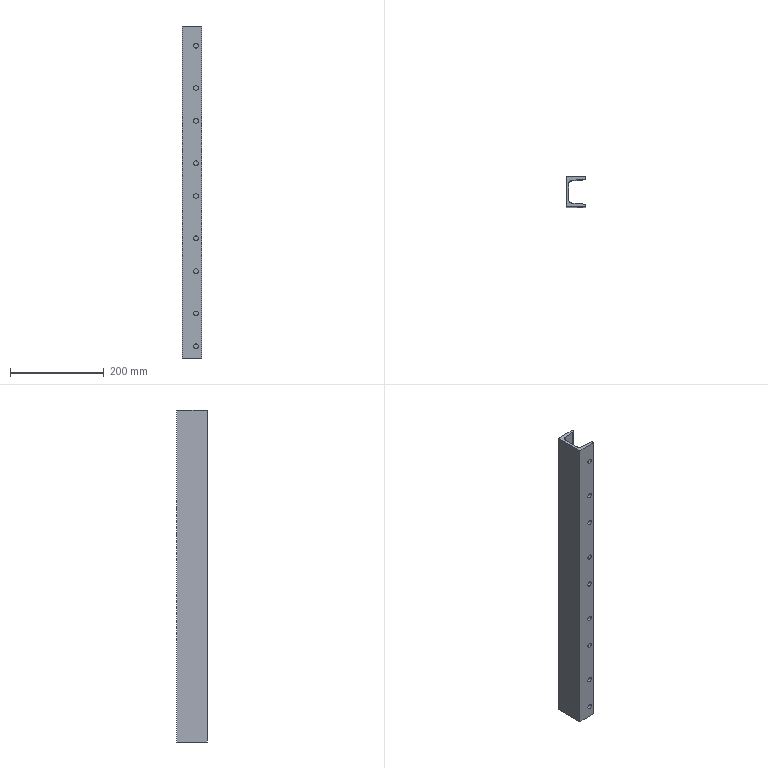Part | STEP file | DIN 1026-1 U 65 1785352380714 | 1 solid | 23 faces | box 42 x 65 x 707.157 mm | volume 633916 mm3 | cylinder 13 | plane 10 | commonest cylinder face diameters 10 x9 8 x2 15 x2
STEP:
#1=CARTESIAN_POINT('',(12.402,-24.312,60.));
#2=VERTEX_POINT('',#1);
#3=CARTESIAN_POINT('',(5.5,-16.836,60.));
#4=VERTEX_POINT('',#3);
#5=CARTESIAN_POINT('',(13.,-16.836,60.));
#6=DIRECTION('',(0.,0.,-1.));
#7=DIRECTION('',(-1.,0.,0.));
#8=AXIS2_PLACEMENT_3D('',#5,#6,#7);
#9=CIRCLE('',#8,7.5);
#10=EDGE_CURVE('',#2,#4,#9,.T.);
#11=ORIENTED_EDGE('',*,*,#10,.F.);
#12=CARTESIAN_POINT('',(38.319,-26.386,60.));
#13=VERTEX_POINT('',#12);
#14=CARTESIAN_POINT('',(15.707,-24.577,60.));
#15=DIRECTION('',(-0.9968,0.07975,0.));
#16=VECTOR('',#15,10.);
#17=LINE('',#14,#16);
#18=EDGE_CURVE('',#13,#2,#17,.T.);
#19=ORIENTED_EDGE('',*,*,#18,.F.);
#20=CARTESIAN_POINT('',(42.,-30.373,60.));
#21=VERTEX_POINT('',#20);
#22=CARTESIAN_POINT('',(38.,-30.373,60.));
#23=DIRECTION('',(0.,0.,1.));
#24=DIRECTION('',(-1.,0.,0.));
#25=AXIS2_PLACEMENT_3D('',#22,#23,#24);
#26=CIRCLE('',#25,4.);
#27=EDGE_CURVE('',#21,#13,#26,.T.);
#28=ORIENTED_EDGE('',*,*,#27,.F.);
#29=CARTESIAN_POINT('',(42.,-32.5,60.));
#30=VERTEX_POINT('',#29);
#31=CARTESIAN_POINT('',(42.,-15.186,60.));
#32=DIRECTION('',(0.,1.,0.));
#33=VECTOR('',#32,10.);
#34=LINE('',#31,#33);
#35=EDGE_CURVE('',#30,#21,#34,.T.);
#36=ORIENTED_EDGE('',*,*,#35,.F.);
#37=CARTESIAN_POINT('',(0.,-32.5,60.));
#38=VERTEX_POINT('',#37);
#39=CARTESIAN_POINT('',(31.5,-32.5,60.));
#40=DIRECTION('',(1.,0.,0.));
#41=VECTOR('',#40,10.);
#42=LINE('',#39,#41);
#43=EDGE_CURVE('',#38,#30,#42,.T.);
#44=ORIENTED_EDGE('',*,*,#43,.F.);
#45=CARTESIAN_POINT('',(0.,32.5,60.));
#46=VERTEX_POINT('',#45);
#47=CARTESIAN_POINT('',(0.,0.,60.));
#48=DIRECTION('',(0.,-1.,0.));
#49=VECTOR('',#48,10.);
#50=LINE('',#47,#49);
#51=EDGE_CURVE('',#46,#38,#50,.T.);
#52=ORIENTED_EDGE('',*,*,#51,.F.);
#53=CARTESIAN_POINT('',(42.,32.5,60.));
#54=VERTEX_POINT('',#53);
#55=CARTESIAN_POINT('',(10.5,32.5,60.));
#56=DIRECTION('',(-1.,0.,0.));
#57=VECTOR('',#56,10.);
#58=LINE('',#55,#57);
#59=EDGE_CURVE('',#54,#46,#58,.T.);
#60=ORIENTED_EDGE('',*,*,#59,.F.);
#61=CARTESIAN_POINT('',(42.,30.373,60.));
#62=VERTEX_POINT('',#61);
#63=CARTESIAN_POINT('',(42.,16.25,60.));
#64=DIRECTION('',(0.,1.,0.));
#65=VECTOR('',#64,10.);
#66=LINE('',#63,#65);
#67=EDGE_CURVE('',#62,#54,#66,.T.);
#68=ORIENTED_EDGE('',*,*,#67,.F.);
#69=CARTESIAN_POINT('',(38.319,26.386,60.));
#70=VERTEX_POINT('',#69);
#71=CARTESIAN_POINT('',(38.,30.373,60.));
#72=DIRECTION('',(0.,0.,1.));
#73=DIRECTION('',(-0.07975,0.9968,0.));
#74=AXIS2_PLACEMENT_3D('',#71,#72,#73);
#75=CIRCLE('',#74,4.);
#76=EDGE_CURVE('',#70,#62,#75,.T.);
#77=ORIENTED_EDGE('',*,*,#76,.F.);
#78=CARTESIAN_POINT('',(12.402,24.312,60.));
#79=VERTEX_POINT('',#78);
#80=CARTESIAN_POINT('',(28.666,25.613,60.));
#81=DIRECTION('',(0.9968,0.07975,0.));
#82=VECTOR('',#81,10.);
#83=LINE('',#80,#82);
#84=EDGE_CURVE('',#79,#70,#83,.T.);
#85=ORIENTED_EDGE('',*,*,#84,.F.);
#86=CARTESIAN_POINT('',(5.5,16.836,60.));
#87=VERTEX_POINT('',#86);
#88=CARTESIAN_POINT('',(13.,16.836,60.));
#89=DIRECTION('',(0.,0.,-1.));
#90=DIRECTION('',(-0.07975,0.9968,0.));
#91=AXIS2_PLACEMENT_3D('',#88,#89,#90);
#92=CIRCLE('',#91,7.5);
#93=EDGE_CURVE('',#87,#79,#92,.T.);
#94=ORIENTED_EDGE('',*,*,#93,.F.);
#95=CARTESIAN_POINT('',(5.5,0.,60.));
#96=DIRECTION('',(0.,1.,0.));
#97=VECTOR('',#96,10.);
#98=LINE('',#95,#97);
#99=EDGE_CURVE('',#4,#87,#98,.T.);
#100=ORIENTED_EDGE('',*,*,#99,.F.);
#101=EDGE_LOOP('',(#11,#19,#28,#36,#44,#52,#60,#68,#77,#85,#94,#100));
#102=FACE_OUTER_BOUND('',#101,.T.);
#103=CARTESIAN_POINT('',(21.,0.,60.));
#104=DIRECTION('',(0.,0.,-1.));
#105=DIRECTION('',(1.,0.,0.));
#106=AXIS2_PLACEMENT_3D('',#103,#104,#105);
#107=PLANE('',#106);
#108=ADVANCED_FACE('',(#102),#107,.T.);
#109=ORIENTED_EDGE('',*,*,#51,.T.);
#110=CARTESIAN_POINT('',(0.,-32.5,767.157));
#111=VERTEX_POINT('',#110);
#112=CARTESIAN_POINT('',(0.,-32.5,0.));
#113=DIRECTION('',(0.,0.,1.));
#114=VECTOR('',#113,10.);
#115=LINE('',#112,#114);
#116=EDGE_CURVE('',#38,#111,#115,.T.);
#117=ORIENTED_EDGE('',*,*,#116,.T.);
#118=CARTESIAN_POINT('',(0.,32.5,767.157));
#119=VERTEX_POINT('',#118);
#120=CARTESIAN_POINT('',(0.,0.,767.157));
#121=DIRECTION('',(0.,1.,0.));
#122=VECTOR('',#121,10.);
#123=LINE('',#120,#122);
#124=EDGE_CURVE('',#111,#119,#123,.T.);
#125=ORIENTED_EDGE('',*,*,#124,.T.);
#126=CARTESIAN_POINT('',(0.,32.5,0.));
#127=DIRECTION('',(0.,0.,1.));
#128=VECTOR('',#127,10.);
#129=LINE('',#126,#128);
#130=EDGE_CURVE('',#46,#119,#129,.T.);
#131=ORIENTED_EDGE('',*,*,#130,.F.);
#132=EDGE_LOOP('',(#109,#117,#125,#131));
#133=FACE_OUTER_BOUND('',#132,.T.);
#134=CARTESIAN_POINT('',(0.,0.,0.));
#135=DIRECTION('',(-1.,0.,0.));
#136=DIRECTION('',(0.,0.,1.));
#137=AXIS2_PLACEMENT_3D('',#134,#135,#136);
#138=PLANE('',#137);
#139=ADVANCED_FACE('',(#133),#138,.T.);
#140=ORIENTED_EDGE('',*,*,#43,.T.);
#141=CARTESIAN_POINT('',(42.,-32.5,767.157));
#142=VERTEX_POINT('',#141);
#143=CARTESIAN_POINT('',(42.,-32.5,0.));
#144=DIRECTION('',(0.,0.,1.));
#145=VECTOR('',#144,10.);
#146=LINE('',#143,#145);
#147=EDGE_CURVE('',#30,#142,#146,.T.);
#148=ORIENTED_EDGE('',*,*,#147,.T.);
#149=CARTESIAN_POINT('',(31.5,-32.5,767.157));
#150=DIRECTION('',(-1.,0.,0.));
#151=VECTOR('',#150,10.);
#152=LINE('',#149,#151);
#153=EDGE_CURVE('',#142,#111,#152,.T.);
#154=ORIENTED_EDGE('',*,*,#153,.T.);
#155=ORIENTED_EDGE('',*,*,#116,.F.);
#156=EDGE_LOOP('',(#140,#148,#154,#155));
#157=FACE_OUTER_BOUND('',#156,.T.);
#158=CARTESIAN_POINT('',(24.5,-32.5,155.));
#159=VERTEX_POINT('',#158);
#160=CARTESIAN_POINT('',(29.5,-32.5,155.));
#161=DIRECTION('',(0.,1.,0.));
#162=DIRECTION('',(1.,0.,0.));
#163=AXIS2_PLACEMENT_3D('',#160,#161,#162);
#164=CIRCLE('',#163,5.);
#165=EDGE_CURVE('',#159,#159,#164,.T.);
#166=ORIENTED_EDGE('',*,*,#165,.T.);
#167=EDGE_LOOP('',(#166));
#168=FACE_BOUND('',#167,.T.);
#169=CARTESIAN_POINT('',(24.5,-32.5,85.));
#170=VERTEX_POINT('',#169);
#171=CARTESIAN_POINT('',(29.5,-32.5,85.));
#172=DIRECTION('',(0.,1.,0.));
#173=DIRECTION('',(1.,0.,0.));
#174=AXIS2_PLACEMENT_3D('',#171,#172,#173);
#175=CIRCLE('',#174,5.);
#176=EDGE_CURVE('',#170,#170,#175,.T.);
#177=ORIENTED_EDGE('',*,*,#176,.T.);
#178=EDGE_LOOP('',(#177));
#179=FACE_BOUND('',#178,.T.);
#180=CARTESIAN_POINT('',(24.5,-32.5,315.));
#181=VERTEX_POINT('',#180);
#182=CARTESIAN_POINT('',(29.5,-32.5,315.));
#183=DIRECTION('',(0.,1.,0.));
#184=DIRECTION('',(1.,0.,0.));
#185=AXIS2_PLACEMENT_3D('',#182,#183,#184);
#186=CIRCLE('',#185,5.);
#187=EDGE_CURVE('',#181,#181,#186,.T.);
#188=ORIENTED_EDGE('',*,*,#187,.T.);
#189=EDGE_LOOP('',(#188));
#190=FACE_BOUND('',#189,.T.);
#191=CARTESIAN_POINT('',(24.5,-32.5,245.));
#192=VERTEX_POINT('',#191);
#193=CARTESIAN_POINT('',(29.5,-32.5,245.));
#194=DIRECTION('',(0.,1.,0.));
#195=DIRECTION('',(1.,0.,0.));
#196=AXIS2_PLACEMENT_3D('',#193,#194,#195);
#197=CIRCLE('',#196,5.);
#198=EDGE_CURVE('',#192,#192,#197,.T.);
#199=ORIENTED_EDGE('',*,*,#198,.T.);
#200=EDGE_LOOP('',(#199));
#201=FACE_BOUND('',#200,.T.);
#202=CARTESIAN_POINT('',(24.5,-32.5,475.));
#203=VERTEX_POINT('',#202);
#204=CARTESIAN_POINT('',(29.5,-32.5,475.));
#205=DIRECTION('',(0.,1.,0.));
#206=DIRECTION('',(1.,0.,0.));
#207=AXIS2_PLACEMENT_3D('',#204,#205,#206);
#208=CIRCLE('',#207,5.);
#209=EDGE_CURVE('',#203,#203,#208,.T.);
#210=ORIENTED_EDGE('',*,*,#209,.T.);
#211=EDGE_LOOP('',(#210));
#212=FACE_BOUND('',#211,.T.);
#213=CARTESIAN_POINT('',(24.5,-32.5,405.));
#214=VERTEX_POINT('',#213);
#215=CARTESIAN_POINT('',(29.5,-32.5,405.));
#216=DIRECTION('',(0.,1.,0.));
#217=DIRECTION('',(1.,0.,0.));
#218=AXIS2_PLACEMENT_3D('',#215,#216,#217);
#219=CIRCLE('',#218,5.);
#220=EDGE_CURVE('',#214,#214,#219,.T.);
#221=ORIENTED_EDGE('',*,*,#220,.T.);
#222=EDGE_LOOP('',(#221));
#223=FACE_BOUND('',#222,.T.);
#224=CARTESIAN_POINT('',(24.5,-32.5,635.));
#225=VERTEX_POINT('',#224);
#226=CARTESIAN_POINT('',(29.5,-32.5,635.));
#227=DIRECTION('',(0.,1.,0.));
#228=DIRECTION('',(1.,0.,0.));
#229=AXIS2_PLACEMENT_3D('',#226,#227,#228);
#230=CIRCLE('',#229,5.);
#231=EDGE_CURVE('',#225,#225,#230,.T.);
#232=ORIENTED_EDGE('',*,*,#231,.T.);
#233=EDGE_LOOP('',(#232));
#234=FACE_BOUND('',#233,.T.);
#235=CARTESIAN_POINT('',(24.5,-32.5,565.));
#236=VERTEX_POINT('',#235);
#237=CARTESIAN_POINT('',(29.5,-32.5,565.));
#238=DIRECTION('',(0.,1.,0.));
#239=DIRECTION('',(1.,0.,0.));
#240=AXIS2_PLACEMENT_3D('',#237,#238,#239);
#241=CIRCLE('',#240,5.);
#242=EDGE_CURVE('',#236,#236,#241,.T.);
#243=ORIENTED_EDGE('',*,*,#242,.T.);
#244=EDGE_LOOP('',(#243));
#245=FACE_BOUND('',#244,.T.);
#246=CARTESIAN_POINT('',(24.5,-32.5,725.));
#247=VERTEX_POINT('',#246);
#248=CARTESIAN_POINT('',(29.5,-32.5,725.));
#249=DIRECTION('',(0.,1.,0.));
#250=DIRECTION('',(1.,0.,0.));
#251=AXIS2_PLACEMENT_3D('',#248,#249,#250);
#252=CIRCLE('',#251,5.);
#253=EDGE_CURVE('',#247,#247,#252,.T.);
#254=ORIENTED_EDGE('',*,*,#253,.T.);
#255=EDGE_LOOP('',(#254));
#256=FACE_BOUND('',#255,.T.);
#257=CARTESIAN_POINT('',(42.,-32.5,0.));
#258=DIRECTION('',(0.,-1.,0.));
#259=DIRECTION('',(0.,0.,-1.));
#260=AXIS2_PLACEMENT_3D('',#257,#258,#259);
#261=PLANE('',#260);
#262=ADVANCED_FACE('',(#157,#168,#179,#190,#201,#212,#223,#234,#245,#256),#261,.T.);
#263=ORIENTED_EDGE('',*,*,#35,.T.);
#264=CARTESIAN_POINT('',(42.,-30.373,767.157));
#265=VERTEX_POINT('',#264);
#266=CARTESIAN_POINT('',(42.,-30.373,0.));
#267=DIRECTION('',(0.,0.,1.));
#268=VECTOR('',#267,10.);
#269=LINE('',#266,#268);
#270=EDGE_CURVE('',#21,#265,#269,.T.);
#271=ORIENTED_EDGE('',*,*,#270,.T.);
#272=CARTESIAN_POINT('',(42.,-15.186,767.157));
#273=DIRECTION('',(0.,-1.,0.));
#274=VECTOR('',#273,10.);
#275=LINE('',#272,#274);
#276=EDGE_CURVE('',#265,#142,#275,.T.);
#277=ORIENTED_EDGE('',*,*,#276,.T.);
#278=ORIENTED_EDGE('',*,*,#147,.F.);
#279=EDGE_LOOP('',(#263,#271,#277,#278));
#280=FACE_OUTER_BOUND('',#279,.T.);
#281=CARTESIAN_POINT('',(42.,-30.373,0.));
#282=DIRECTION('',(1.,0.,0.));
#283=DIRECTION('',(0.,0.,-1.));
#284=AXIS2_PLACEMENT_3D('',#281,#282,#283);
#285=PLANE('',#284);
#286=ADVANCED_FACE('',(#280),#285,.T.);
#287=ORIENTED_EDGE('',*,*,#27,.T.);
#288=CARTESIAN_POINT('',(38.319,-26.386,767.157));
#289=VERTEX_POINT('',#288);
#290=CARTESIAN_POINT('',(38.319,-26.386,0.));
#291=DIRECTION('',(0.,0.,1.));
#292=VECTOR('',#291,10.);
#293=LINE('',#290,#292);
#294=EDGE_CURVE('',#13,#289,#293,.T.);
#295=ORIENTED_EDGE('',*,*,#294,.T.);
#296=CARTESIAN_POINT('',(38.,-30.373,767.157));
#297=DIRECTION('',(0.,0.,-1.));
#298=DIRECTION('',(-1.,0.,0.));
#299=AXIS2_PLACEMENT_3D('',#296,#297,#298);
#300=CIRCLE('',#299,4.);
#301=EDGE_CURVE('',#289,#265,#300,.T.);
#302=ORIENTED_EDGE('',*,*,#301,.T.);
#303=ORIENTED_EDGE('',*,*,#270,.F.);
#304=EDGE_LOOP('',(#287,#295,#302,#303));
#305=FACE_OUTER_BOUND('',#304,.T.);
#306=CARTESIAN_POINT('',(38.,-30.373,0.));
#307=DIRECTION('',(0.,0.,1.));
#308=DIRECTION('',(-1.,0.,0.));
#309=AXIS2_PLACEMENT_3D('',#306,#307,#308);
#310=CYLINDRICAL_SURFACE('',#309,4.);
#311=ADVANCED_FACE('',(#305),#310,.T.);
#312=ORIENTED_EDGE('',*,*,#18,.T.);
#313=CARTESIAN_POINT('',(12.402,-24.312,767.157));
#314=VERTEX_POINT('',#313);
#315=CARTESIAN_POINT('',(12.402,-24.312,0.));
#316=DIRECTION('',(0.,0.,1.));
#317=VECTOR('',#316,10.);
#318=LINE('',#315,#317);
#319=EDGE_CURVE('',#2,#314,#318,.T.);
#320=ORIENTED_EDGE('',*,*,#319,.T.);
#321=CARTESIAN_POINT('',(15.707,-24.577,767.157));
#322=DIRECTION('',(0.9968,-0.07975,0.));
#323=VECTOR('',#322,10.);
#324=LINE('',#321,#323);
#325=EDGE_CURVE('',#314,#289,#324,.T.);
#326=ORIENTED_EDGE('',*,*,#325,.T.);
#327=ORIENTED_EDGE('',*,*,#294,.F.);
#328=EDGE_LOOP('',(#312,#320,#326,#327));
#329=FACE_OUTER_BOUND('',#328,.T.);
#330=CARTESIAN_POINT('',(24.5,-25.28,155.));
#331=VERTEX_POINT('',#330);
#332=CARTESIAN_POINT('',(29.5,-25.68,155.));
#333=DIRECTION('',(-0.07975,-0.9968,0.));
#334=DIRECTION('',(0.9968,-0.07975,0.));
#335=AXIS2_PLACEMENT_3D('',#332,#333,#334);
#336=ELLIPSE('',#335,5.016,5.);
#337=EDGE_CURVE('',#331,#331,#336,.T.);
#338=ORIENTED_EDGE('',*,*,#337,.T.);
#339=EDGE_LOOP('',(#338));
#340=FACE_BOUND('',#339,.T.);
#341=CARTESIAN_POINT('',(24.5,-25.28,85.));
#342=VERTEX_POINT('',#341);
#343=CARTESIAN_POINT('',(29.5,-25.68,85.));
#344=DIRECTION('',(-0.07975,-0.9968,0.));
#345=DIRECTION('',(0.9968,-0.07975,0.));
#346=AXIS2_PLACEMENT_3D('',#343,#344,#345);
#347=ELLIPSE('',#346,5.016,5.);
#348=EDGE_CURVE('',#342,#342,#347,.T.);
#349=ORIENTED_EDGE('',*,*,#348,.T.);
#350=EDGE_LOOP('',(#349));
#351=FACE_BOUND('',#350,.T.);
#352=CARTESIAN_POINT('',(24.5,-25.28,315.));
#353=VERTEX_POINT('',#352);
#354=CARTESIAN_POINT('',(29.5,-25.68,315.));
#355=DIRECTION('',(-0.07975,-0.9968,0.));
#356=DIRECTION('',(0.9968,-0.07975,0.));
#357=AXIS2_PLACEMENT_3D('',#354,#355,#356);
#358=ELLIPSE('',#357,5.016,5.);
#359=EDGE_CURVE('',#353,#353,#358,.T.);
#360=ORIENTED_EDGE('',*,*,#359,.T.);
#361=EDGE_LOOP('',(#360));
#362=FACE_BOUND('',#361,.T.);
#363=CARTESIAN_POINT('',(24.5,-25.28,245.));
#364=VERTEX_POINT('',#363);
#365=CARTESIAN_POINT('',(29.5,-25.68,245.));
#366=DIRECTION('',(-0.07975,-0.9968,0.));
#367=DIRECTION('',(0.9968,-0.07975,0.));
#368=AXIS2_PLACEMENT_3D('',#365,#366,#367);
#369=ELLIPSE('',#368,5.016,5.);
#370=EDGE_CURVE('',#364,#364,#369,.T.);
#371=ORIENTED_EDGE('',*,*,#370,.T.);
#372=EDGE_LOOP('',(#371));
#373=FACE_BOUND('',#372,.T.);
#374=CARTESIAN_POINT('',(24.5,-25.28,475.));
#375=VERTEX_POINT('',#374);
#376=CARTESIAN_POINT('',(29.5,-25.68,475.));
#377=DIRECTION('',(-0.07975,-0.9968,0.));
#378=DIRECTION('',(0.9968,-0.07975,0.));
#379=AXIS2_PLACEMENT_3D('',#376,#377,#378);
#380=ELLIPSE('',#379,5.016,5.);
#381=EDGE_CURVE('',#375,#375,#380,.T.);
#382=ORIENTED_EDGE('',*,*,#381,.T.);
#383=EDGE_LOOP('',(#382));
#384=FACE_BOUND('',#383,.T.);
#385=CARTESIAN_POINT('',(24.5,-25.28,405.));
#386=VERTEX_POINT('',#385);
#387=CARTESIAN_POINT('',(29.5,-25.68,405.));
#388=DIRECTION('',(-0.07975,-0.9968,0.));
#389=DIRECTION('',(0.9968,-0.07975,0.));
#390=AXIS2_PLACEMENT_3D('',#387,#388,#389);
#391=ELLIPSE('',#390,5.016,5.);
#392=EDGE_CURVE('',#386,#386,#391,.T.);
#393=ORIENTED_EDGE('',*,*,#392,.T.);
#394=EDGE_LOOP('',(#393));
#395=FACE_BOUND('',#394,.T.);
#396=CARTESIAN_POINT('',(24.5,-25.28,635.));
#397=VERTEX_POINT('',#396);
#398=CARTESIAN_POINT('',(29.5,-25.68,635.));
#399=DIRECTION('',(-0.07975,-0.9968,0.));
#400=DIRECTION('',(0.9968,-0.07975,0.));
#401=AXIS2_PLACEMENT_3D('',#398,#399,#400);
#402=ELLIPSE('',#401,5.016,5.);
#403=EDGE_CURVE('',#397,#397,#402,.T.);
#404=ORIENTED_EDGE('',*,*,#403,.T.);
#405=EDGE_LOOP('',(#404));
#406=FACE_BOUND('',#405,.T.);
#407=CARTESIAN_POINT('',(24.5,-25.28,565.));
#408=VERTEX_POINT('',#407);
#409=CARTESIAN_POINT('',(29.5,-25.68,565.));
#410=DIRECTION('',(-0.07975,-0.9968,0.));
#411=DIRECTION('',(0.9968,-0.07975,0.));
#412=AXIS2_PLACEMENT_3D('',#409,#410,#411);
#413=ELLIPSE('',#412,5.016,5.);
#414=EDGE_CURVE('',#408,#408,#413,.T.);
#415=ORIENTED_EDGE('',*,*,#414,.T.);
#416=EDGE_LOOP('',(#415));
#417=FACE_BOUND('',#416,.T.);
#418=CARTESIAN_POINT('',(24.5,-25.28,725.));
#419=VERTEX_POINT('',#418);
#420=CARTESIAN_POINT('',(29.5,-25.68,725.));
#421=DIRECTION('',(-0.07975,-0.9968,0.));
#422=DIRECTION('',(0.9968,-0.07975,0.));
#423=AXIS2_PLACEMENT_3D('',#420,#421,#422);
#424=ELLIPSE('',#423,5.016,5.);
#425=EDGE_CURVE('',#419,#419,#424,.T.);
#426=ORIENTED_EDGE('',*,*,#425,.T.);
#427=EDGE_LOOP('',(#426));
#428=FACE_BOUND('',#427,.T.);
#429=CARTESIAN_POINT('',(12.402,-24.312,0.));
#430=DIRECTION('',(0.07975,0.9968,0.));
#431=DIRECTION('',(0.,0.,1.));
#432=AXIS2_PLACEMENT_3D('',#429,#430,#431);
#433=PLANE('',#432);
#434=ADVANCED_FACE('',(#329,#340,#351,#362,#373,#384,#395,#406,#417,#428),#433,.T.);
#435=ORIENTED_EDGE('',*,*,#10,.T.);
#436=CARTESIAN_POINT('',(5.5,-16.836,767.157));
#437=VERTEX_POINT('',#436);
#438=CARTESIAN_POINT('',(5.5,-16.836,0.));
#439=DIRECTION('',(0.,0.,1.));
#440=VECTOR('',#439,10.);
#441=LINE('',#438,#440);
#442=EDGE_CURVE('',#4,#437,#441,.T.);
#443=ORIENTED_EDGE('',*,*,#442,.T.);
#444=CARTESIAN_POINT('',(13.,-16.836,767.157));
#445=DIRECTION('',(0.,0.,1.));
#446=DIRECTION('',(-1.,0.,0.));
#447=AXIS2_PLACEMENT_3D('',#444,#445,#446);
#448=CIRCLE('',#447,7.5);
#449=EDGE_CURVE('',#437,#314,#448,.T.);
#450=ORIENTED_EDGE('',*,*,#449,.T.);
#451=ORIENTED_EDGE('',*,*,#319,.F.);
#452=EDGE_LOOP('',(#435,#443,#450,#451));
#453=FACE_OUTER_BOUND('',#452,.T.);
#454=CARTESIAN_POINT('',(13.,-16.836,0.));
#455=DIRECTION('',(0.,0.,1.));
#456=DIRECTION('',(-1.,0.,0.));
#457=AXIS2_PLACEMENT_3D('',#454,#455,#456);
#458=CYLINDRICAL_SURFACE('',#457,7.5);
#459=ADVANCED_FACE('',(#453),#458,.F.);
#460=ORIENTED_EDGE('',*,*,#253,.F.);
#461=CARTESIAN_POINT('',(24.5,-32.5,725.));
#462=DIRECTION('',(0.,1.,0.));
#463=VECTOR('',#462,5.);
#464=LINE('',#461,#463);
#465=EDGE_CURVE('',#247,#419,#464,.T.);
#466=ORIENTED_EDGE('',*,*,#465,.T.);
#467=ORIENTED_EDGE('',*,*,#425,.F.);
#468=ORIENTED_EDGE('',*,*,#465,.F.);
#469=EDGE_LOOP('',(#460,#466,#467,#468));
#470=FACE_OUTER_BOUND('',#469,.T.);
#471=CARTESIAN_POINT('',(29.5,-32.5,725.));
#472=DIRECTION('',(0.,1.,0.));
#473=DIRECTION('',(1.,0.,0.));
#474=AXIS2_PLACEMENT_3D('',#471,#472,#473);
#475=CYLINDRICAL_SURFACE('',#474,5.);
#476=ADVANCED_FACE('',(#470),#475,.F.);
#477=ORIENTED_EDGE('',*,*,#242,.F.);
#478=CARTESIAN_POINT('',(24.5,-32.5,565.));
#479=DIRECTION('',(0.,1.,0.));
#480=VECTOR('',#479,5.);
#481=LINE('',#478,#480);
#482=EDGE_CURVE('',#236,#408,#481,.T.);
#483=ORIENTED_EDGE('',*,*,#482,.T.);
#484=ORIENTED_EDGE('',*,*,#414,.F.);
#485=ORIENTED_EDGE('',*,*,#482,.F.);
#486=EDGE_LOOP('',(#477,#483,#484,#485));
#487=FACE_OUTER_BOUND('',#486,.T.);
#488=CARTESIAN_POINT('',(29.5,-32.5,565.));
#489=DIRECTION('',(0.,1.,0.));
#490=DIRECTION('',(1.,0.,0.));
#491=AXIS2_PLACEMENT_3D('',#488,#489,#490);
#492=CYLINDRICAL_SURFACE('',#491,5.);
#493=ADVANCED_FACE('',(#487),#492,.F.);
#494=ORIENTED_EDGE('',*,*,#231,.F.);
#495=CARTESIAN_POINT('',(24.5,-32.5,635.));
#496=DIRECTION('',(0.,1.,0.));
#497=VECTOR('',#496,5.);
#498=LINE('',#495,#497);
#499=EDGE_CURVE('',#225,#397,#498,.T.);
#500=ORIENTED_EDGE('',*,*,#499,.T.);
#501=ORIENTED_EDGE('',*,*,#403,.F.);
#502=ORIENTED_EDGE('',*,*,#499,.F.);
#503=EDGE_LOOP('',(#494,#500,#501,#502));
#504=FACE_OUTER_BOUND('',#503,.T.);
#505=CARTESIAN_POINT('',(29.5,-32.5,635.));
#506=DIRECTION('',(0.,1.,0.));
#507=DIRECTION('',(1.,0.,0.));
#508=AXIS2_PLACEMENT_3D('',#505,#506,#507);
#509=CYLINDRICAL_SURFACE('',#508,5.);
#510=ADVANCED_FACE('',(#504),#509,.F.);
#511=ORIENTED_EDGE('',*,*,#220,.F.);
#512=CARTESIAN_POINT('',(24.5,-32.5,405.));
#513=DIRECTION('',(0.,1.,0.));
#514=VECTOR('',#513,5.);
#515=LINE('',#512,#514);
#516=EDGE_CURVE('',#214,#386,#515,.T.);
#517=ORIENTED_EDGE('',*,*,#516,.T.);
#518=ORIENTED_EDGE('',*,*,#392,.F.);
#519=ORIENTED_EDGE('',*,*,#516,.F.);
#520=EDGE_LOOP('',(#511,#517,#518,#519));
#521=FACE_OUTER_BOUND('',#520,.T.);
#522=CARTESIAN_POINT('',(29.5,-32.5,405.));
#523=DIRECTION('',(0.,1.,0.));
#524=DIRECTION('',(1.,0.,0.));
#525=AXIS2_PLACEMENT_3D('',#522,#523,#524);
#526=CYLINDRICAL_SURFACE('',#525,5.);
#527=ADVANCED_FACE('',(#521),#526,.F.);
#528=ORIENTED_EDGE('',*,*,#209,.F.);
#529=CARTESIAN_POINT('',(24.5,-32.5,475.));
#530=DIRECTION('',(0.,1.,0.));
#531=VECTOR('',#530,5.);
#532=LINE('',#529,#531);
#533=EDGE_CURVE('',#203,#375,#532,.T.);
#534=ORIENTED_EDGE('',*,*,#533,.T.);
#535=ORIENTED_EDGE('',*,*,#381,.F.);
#536=ORIENTED_EDGE('',*,*,#533,.F.);
#537=EDGE_LOOP('',(#528,#534,#535,#536));
#538=FACE_OUTER_BOUND('',#537,.T.);
#539=CARTESIAN_POINT('',(29.5,-32.5,475.));
#540=DIRECTION('',(0.,1.,0.));
#541=DIRECTION('',(1.,0.,0.));
#542=AXIS2_PLACEMENT_3D('',#539,#540,#541);
#543=CYLINDRICAL_SURFACE('',#542,5.);
#544=ADVANCED_FACE('',(#538),#543,.F.);
#545=ORIENTED_EDGE('',*,*,#198,.F.);
#546=CARTESIAN_POINT('',(24.5,-32.5,245.));
#547=DIRECTION('',(0.,1.,0.));
#548=VECTOR('',#547,5.);
#549=LINE('',#546,#548);
#550=EDGE_CURVE('',#192,#364,#549,.T.);
#551=ORIENTED_EDGE('',*,*,#550,.T.);
#552=ORIENTED_EDGE('',*,*,#370,.F.);
#553=ORIENTED_EDGE('',*,*,#550,.F.);
#554=EDGE_LOOP('',(#545,#551,#552,#553));
#555=FACE_OUTER_BOUND('',#554,.T.);
#556=CARTESIAN_POINT('',(29.5,-32.5,245.));
#557=DIRECTION('',(0.,1.,0.));
#558=DIRECTION('',(1.,0.,0.));
#559=AXIS2_PLACEMENT_3D('',#556,#557,#558);
#560=CYLINDRICAL_SURFACE('',#559,5.);
#561=ADVANCED_FACE('',(#555),#560,.F.);
#562=ORIENTED_EDGE('',*,*,#187,.F.);
#563=CARTESIAN_POINT('',(24.5,-32.5,315.));
#564=DIRECTION('',(0.,1.,0.));
#565=VECTOR('',#564,5.);
#566=LINE('',#563,#565);
#567=EDGE_CURVE('',#181,#353,#566,.T.);
#568=ORIENTED_EDGE('',*,*,#567,.T.);
#569=ORIENTED_EDGE('',*,*,#359,.F.);
#570=ORIENTED_EDGE('',*,*,#567,.F.);
#571=EDGE_LOOP('',(#562,#568,#569,#570));
#572=FACE_OUTER_BOUND('',#571,.T.);
#573=CARTESIAN_POINT('',(29.5,-32.5,315.));
#574=DIRECTION('',(0.,1.,0.));
#575=DIRECTION('',(1.,0.,0.));
#576=AXIS2_PLACEMENT_3D('',#573,#574,#575);
#577=CYLINDRICAL_SURFACE('',#576,5.);
#578=ADVANCED_FACE('',(#572),#577,.F.);
#579=ORIENTED_EDGE('',*,*,#176,.F.);
#580=CARTESIAN_POINT('',(24.5,-32.5,85.));
#581=DIRECTION('',(0.,1.,0.));
#582=VECTOR('',#581,5.);
#583=LINE('',#580,#582);
#584=EDGE_CURVE('',#170,#342,#583,.T.);
#585=ORIENTED_EDGE('',*,*,#584,.T.);
#586=ORIENTED_EDGE('',*,*,#348,.F.);
#587=ORIENTED_EDGE('',*,*,#584,.F.);
#588=EDGE_LOOP('',(#579,#585,#586,#587));
#589=FACE_OUTER_BOUND('',#588,.T.);
#590=CARTESIAN_POINT('',(29.5,-32.5,85.));
#591=DIRECTION('',(0.,1.,0.));
#592=DIRECTION('',(1.,0.,0.));
#593=AXIS2_PLACEMENT_3D('',#590,#591,#592);
#594=CYLINDRICAL_SURFACE('',#593,5.);
#595=ADVANCED_FACE('',(#589),#594,.F.);
#596=ORIENTED_EDGE('',*,*,#165,.F.);
#597=CARTESIAN_POINT('',(24.5,-32.5,155.));
#598=DIRECTION('',(0.,1.,0.));
#599=VECTOR('',#598,5.);
#600=LINE('',#597,#599);
#601=EDGE_CURVE('',#159,#331,#600,.T.);
#602=ORIENTED_EDGE('',*,*,#601,.T.);
#603=ORIENTED_EDGE('',*,*,#337,.F.);
#604=ORIENTED_EDGE('',*,*,#601,.F.);
#605=EDGE_LOOP('',(#596,#602,#603,#604));
#606=FACE_OUTER_BOUND('',#605,.T.);
#607=CARTESIAN_POINT('',(29.5,-32.5,155.));
#608=DIRECTION('',(0.,1.,0.));
#609=DIRECTION('',(1.,0.,0.));
#610=AXIS2_PLACEMENT_3D('',#607,#608,#609);
#611=CYLINDRICAL_SURFACE('',#610,5.);
#612=ADVANCED_FACE('',(#606),#611,.F.);
#613=ORIENTED_EDGE('',*,*,#59,.T.);
#614=ORIENTED_EDGE('',*,*,#130,.T.);
#615=CARTESIAN_POINT('',(42.,32.5,767.157));
#616=VERTEX_POINT('',#615);
#617=CARTESIAN_POINT('',(10.5,32.5,767.157));
#618=DIRECTION('',(1.,0.,0.));
#619=VECTOR('',#618,10.);
#620=LINE('',#617,#619);
#621=EDGE_CURVE('',#119,#616,#620,.T.);
#622=ORIENTED_EDGE('',*,*,#621,.T.);
#623=CARTESIAN_POINT('',(42.,32.5,0.));
#624=DIRECTION('',(0.,0.,1.));
#625=VECTOR('',#624,10.);
#626=LINE('',#623,#625);
#627=EDGE_CURVE('',#54,#616,#626,.T.);
#628=ORIENTED_EDGE('',*,*,#627,.F.);
#629=EDGE_LOOP('',(#613,#614,#622,#628));
#630=FACE_OUTER_BOUND('',#629,.T.);
#631=CARTESIAN_POINT('',(0.,32.5,0.));
#632=DIRECTION('',(0.,1.,0.));
#633=DIRECTION('',(0.,0.,1.));
#634=AXIS2_PLACEMENT_3D('',#631,#632,#633);
#635=PLANE('',#634);
#636=ADVANCED_FACE('',(#630),#635,.T.);
#637=ORIENTED_EDGE('',*,*,#67,.T.);
#638=ORIENTED_EDGE('',*,*,#627,.T.);
#639=CARTESIAN_POINT('',(42.,30.373,767.157));
#640=VERTEX_POINT('',#639);
#641=CARTESIAN_POINT('',(42.,16.25,767.157));
#642=DIRECTION('',(0.,-1.,0.));
#643=VECTOR('',#642,10.);
#644=LINE('',#641,#643);
#645=EDGE_CURVE('',#616,#640,#644,.T.);
#646=ORIENTED_EDGE('',*,*,#645,.T.);
#647=CARTESIAN_POINT('',(42.,30.373,0.));
#648=DIRECTION('',(0.,0.,1.));
#649=VECTOR('',#648,10.);
#650=LINE('',#647,#649);
#651=EDGE_CURVE('',#62,#640,#650,.T.);
#652=ORIENTED_EDGE('',*,*,#651,.F.);
#653=EDGE_LOOP('',(#637,#638,#646,#652));
#654=FACE_OUTER_BOUND('',#653,.T.);
#655=CARTESIAN_POINT('',(42.,32.5,0.));
#656=DIRECTION('',(1.,0.,0.));
#657=DIRECTION('',(0.,0.,-1.));
#658=AXIS2_PLACEMENT_3D('',#655,#656,#657);
#659=PLANE('',#658);
#660=ADVANCED_FACE('',(#654),#659,.T.);
#661=ORIENTED_EDGE('',*,*,#76,.T.);
#662=ORIENTED_EDGE('',*,*,#651,.T.);
#663=CARTESIAN_POINT('',(38.319,26.386,767.157));
#664=VERTEX_POINT('',#663);
#665=CARTESIAN_POINT('',(38.,30.373,767.157));
#666=DIRECTION('',(0.,0.,-1.));
#667=DIRECTION('',(-0.07975,0.9968,0.));
#668=AXIS2_PLACEMENT_3D('',#665,#666,#667);
#669=CIRCLE('',#668,4.);
#670=EDGE_CURVE('',#640,#664,#669,.T.);
#671=ORIENTED_EDGE('',*,*,#670,.T.);
#672=CARTESIAN_POINT('',(38.319,26.386,0.));
#673=DIRECTION('',(0.,0.,1.));
#674=VECTOR('',#673,10.);
#675=LINE('',#672,#674);
#676=EDGE_CURVE('',#70,#664,#675,.T.);
#677=ORIENTED_EDGE('',*,*,#676,.F.);
#678=EDGE_LOOP('',(#661,#662,#671,#677));
#679=FACE_OUTER_BOUND('',#678,.T.);
#680=CARTESIAN_POINT('',(38.,30.373,0.));
#681=DIRECTION('',(0.,0.,1.));
#682=DIRECTION('',(-0.07975,0.9968,0.));
#683=AXIS2_PLACEMENT_3D('',#680,#681,#682);
#684=CYLINDRICAL_SURFACE('',#683,4.);
#685=ADVANCED_FACE('',(#679),#684,.T.);
#686=ORIENTED_EDGE('',*,*,#84,.T.);
#687=ORIENTED_EDGE('',*,*,#676,.T.);
#688=CARTESIAN_POINT('',(12.402,24.312,767.157));
#689=VERTEX_POINT('',#688);
#690=CARTESIAN_POINT('',(28.666,25.613,767.157));
#691=DIRECTION('',(-0.9968,-0.07975,0.));
#692=VECTOR('',#691,10.);
#693=LINE('',#690,#692);
#694=EDGE_CURVE('',#664,#689,#693,.T.);
#695=ORIENTED_EDGE('',*,*,#694,.T.);
#696=CARTESIAN_POINT('',(12.402,24.312,0.));
#697=DIRECTION('',(0.,0.,1.));
#698=VECTOR('',#697,10.);
#699=LINE('',#696,#698);
#700=EDGE_CURVE('',#79,#689,#699,.T.);
#701=ORIENTED_EDGE('',*,*,#700,.F.);
#702=EDGE_LOOP('',(#686,#687,#695,#701));
#703=FACE_OUTER_BOUND('',#702,.T.);
#704=CARTESIAN_POINT('',(38.319,26.386,0.));
#705=DIRECTION('',(0.07975,-0.9968,0.));
#706=DIRECTION('',(0.,0.,-1.));
#707=AXIS2_PLACEMENT_3D('',#704,#705,#706);
#708=PLANE('',#707);
#709=ADVANCED_FACE('',(#703),#708,.T.);
#710=ORIENTED_EDGE('',*,*,#93,.T.);
#711=ORIENTED_EDGE('',*,*,#700,.T.);
#712=CARTESIAN_POINT('',(5.5,16.836,767.157));
#713=VERTEX_POINT('',#712);
#714=CARTESIAN_POINT('',(13.,16.836,767.157));
#715=DIRECTION('',(0.,0.,1.));
#716=DIRECTION('',(-0.07975,0.9968,0.));
#717=AXIS2_PLACEMENT_3D('',#714,#715,#716);
#718=CIRCLE('',#717,7.5);
#719=EDGE_CURVE('',#689,#713,#718,.T.);
#720=ORIENTED_EDGE('',*,*,#719,.T.);
#721=CARTESIAN_POINT('',(5.5,16.836,0.));
#722=DIRECTION('',(0.,0.,1.));
#723=VECTOR('',#722,10.);
#724=LINE('',#721,#723);
#725=EDGE_CURVE('',#87,#713,#724,.T.);
#726=ORIENTED_EDGE('',*,*,#725,.F.);
#727=EDGE_LOOP('',(#710,#711,#720,#726));
#728=FACE_OUTER_BOUND('',#727,.T.);
#729=CARTESIAN_POINT('',(13.,16.836,0.));
#730=DIRECTION('',(0.,0.,1.));
#731=DIRECTION('',(-0.07975,0.9968,0.));
#732=AXIS2_PLACEMENT_3D('',#729,#730,#731);
#733=CYLINDRICAL_SURFACE('',#732,7.5);
#734=ADVANCED_FACE('',(#728),#733,.F.);
#735=ORIENTED_EDGE('',*,*,#99,.T.);
#736=ORIENTED_EDGE('',*,*,#725,.T.);
#737=CARTESIAN_POINT('',(5.5,0.,767.157));
#738=DIRECTION('',(0.,-1.,0.));
#739=VECTOR('',#738,10.);
#740=LINE('',#737,#739);
#741=EDGE_CURVE('',#713,#437,#740,.T.);
#742=ORIENTED_EDGE('',*,*,#741,.T.);
#743=ORIENTED_EDGE('',*,*,#442,.F.);
#744=EDGE_LOOP('',(#735,#736,#742,#743));
#745=FACE_OUTER_BOUND('',#744,.T.);
#746=CARTESIAN_POINT('',(5.5,0.,0.));
#747=DIRECTION('',(1.,0.,0.));
#748=DIRECTION('',(0.,0.,-1.));
#749=AXIS2_PLACEMENT_3D('',#746,#747,#748);
#750=PLANE('',#749);
#751=ADVANCED_FACE('',(#745),#750,.T.);
#752=ORIENTED_EDGE('',*,*,#621,.F.);
#753=ORIENTED_EDGE('',*,*,#124,.F.);
#754=ORIENTED_EDGE('',*,*,#153,.F.);
#755=ORIENTED_EDGE('',*,*,#276,.F.);
#756=ORIENTED_EDGE('',*,*,#301,.F.);
#757=ORIENTED_EDGE('',*,*,#325,.F.);
#758=ORIENTED_EDGE('',*,*,#449,.F.);
#759=ORIENTED_EDGE('',*,*,#741,.F.);
#760=ORIENTED_EDGE('',*,*,#719,.F.);
#761=ORIENTED_EDGE('',*,*,#694,.F.);
#762=ORIENTED_EDGE('',*,*,#670,.F.);
#763=ORIENTED_EDGE('',*,*,#645,.F.);
#764=EDGE_LOOP('',(#752,#753,#754,#755,#756,#757,#758,#759,#760,#761,#762,#763));
#765=FACE_OUTER_BOUND('',#764,.T.);
#766=CARTESIAN_POINT('',(21.,0.,767.157));
#767=DIRECTION('',(0.,0.,1.));
#768=DIRECTION('',(1.,0.,0.));
#769=AXIS2_PLACEMENT_3D('',#766,#767,#768);
#770=PLANE('',#769);
#771=ADVANCED_FACE('',(#765),#770,.T.);
#772=CLOSED_SHELL('',(#108,#139,#262,#286,#311,#434,#459,#476,#493,#510,#527,#544,#561,#578,#595,#612,#636,#660,#685,#709,#734,#751,#771));
#773=MANIFOLD_SOLID_BREP('',#772);
#774=(LENGTH_UNIT()NAMED_UNIT(*)SI_UNIT(.MILLI.,.METRE.));
#775=UNCERTAINTY_MEASURE_WITH_UNIT(LENGTH_MEASURE(0.01),#774,'','');
#776=(NAMED_UNIT(*)PLANE_ANGLE_UNIT()SI_UNIT($,.RADIAN.));
#777=(NAMED_UNIT(*)SI_UNIT($,.STERADIAN.)SOLID_ANGLE_UNIT());
#778=(GEOMETRIC_REPRESENTATION_CONTEXT(3)GLOBAL_UNCERTAINTY_ASSIGNED_CONTEXT((#775))GLOBAL_UNIT_ASSIGNED_CONTEXT((#774,#776,#777))REPRESENTATION_CONTEXT('',''));
#779=ADVANCED_BREP_SHAPE_REPRESENTATION('',(#773),#778);